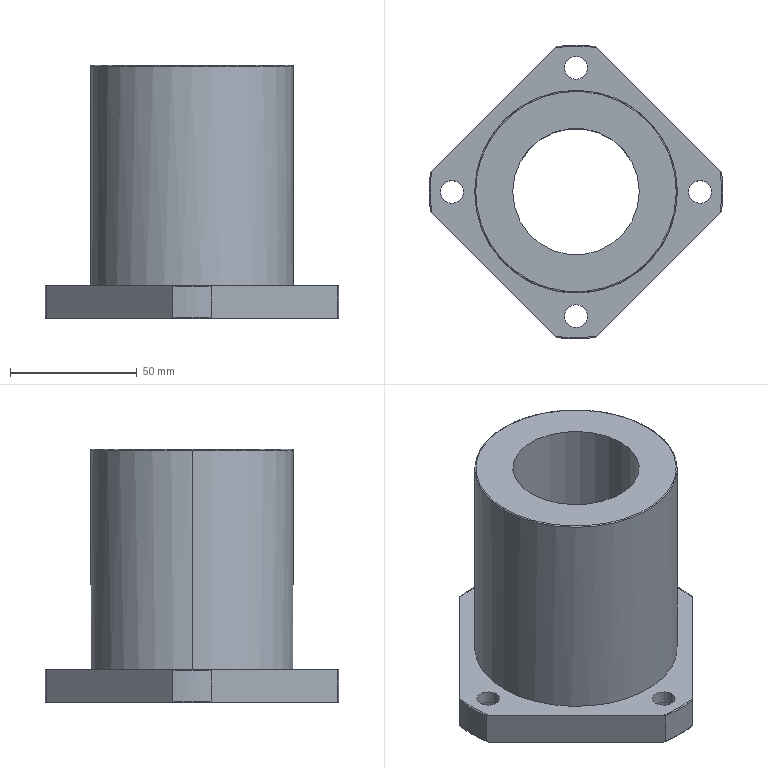Part | SolidWorks | features BaseBody 1 | 1 solid | 48 faces | box 116 x 116 x 100 mm | volume 342037 mm3 | cylinder 25 | spline 12 | plane 11 | commonest cylinder face diameters 9 x8 14 x8 116 x5 50 x2 80 x2